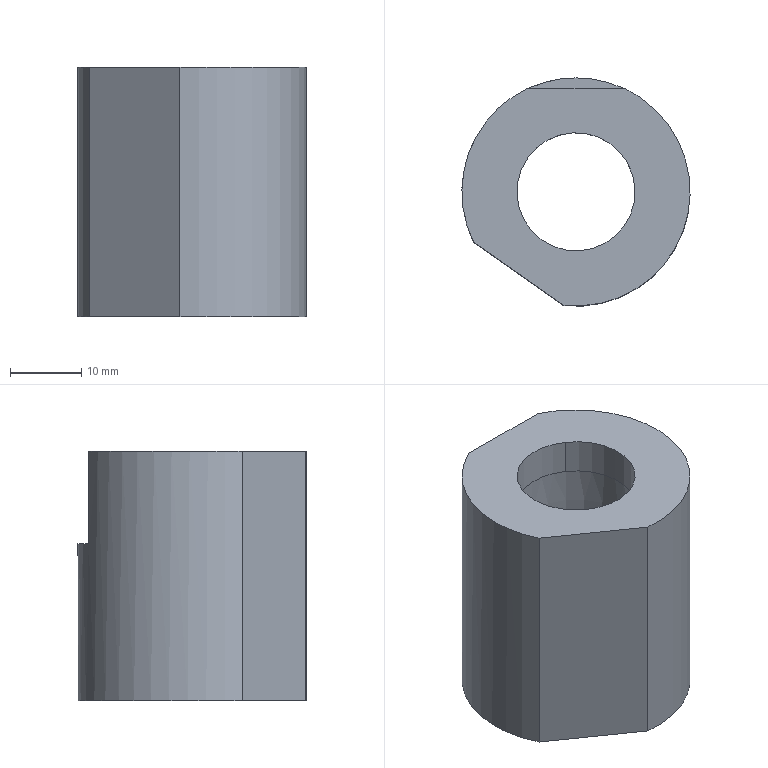Part | STEP file | 1_id4534_x_t | 1 solid | 9 faces | box 32 x 32 x 35 mm | volume 19058 mm3 | plane 5 | cylinder 3 | cone 1 | commonest cylinder face diameters 16.57 x2 32 x1
STEP:
#1=CARTESIAN_POINT('',(3362.815,59.589,-35.));
#2=VERTEX_POINT('',#1);
#3=CARTESIAN_POINT('',(3350.125,68.475,-35.));
#4=VERTEX_POINT('',#3);
#5=CARTESIAN_POINT('',(3356.47,64.032,-35.));
#6=DIRECTION('',(-0.8192,0.5736,0.));
#7=VECTOR('',#6,1.);
#8=LINE('',#5,#7);
#9=EDGE_CURVE('',#2,#4,#8,.T.);
#10=ORIENTED_EDGE('',*,*,#9,.T.);
#11=CARTESIAN_POINT('',(3364.5,75.5,-35.));
#12=DIRECTION('',(0.,0.,1.));
#13=DIRECTION('',(-1.,0.,0.));
#14=AXIS2_PLACEMENT_3D('',#11,#12,#13);
#15=CIRCLE('',#14,16.);
#16=EDGE_CURVE('',#2,#4,#15,.T.);
#17=ORIENTED_EDGE('',*,*,#16,.F.);
#18=EDGE_LOOP('',(#10,#17));
#19=FACE_BOUND('',#18,.T.);
#20=CARTESIAN_POINT('',(3355.43,75.5,-35.));
#21=VERTEX_POINT('',#20);
#22=CARTESIAN_POINT('',(3364.5,75.5,-35.));
#23=DIRECTION('',(0.,0.,1.));
#24=DIRECTION('',(-1.,0.,0.));
#25=AXIS2_PLACEMENT_3D('',#22,#23,#24);
#26=CIRCLE('',#25,9.071);
#27=EDGE_CURVE('',#21,#21,#26,.T.);
#28=ORIENTED_EDGE('',*,*,#27,.T.);
#29=EDGE_LOOP('',(#28));
#30=FACE_BOUND('',#29,.T.);
#31=CARTESIAN_POINT('',(3368.085,80.62,-35.));
#32=DIRECTION('',(0.,0.,-1.));
#33=DIRECTION('',(0.5736,0.8192,0.));
#34=AXIS2_PLACEMENT_3D('',#31,#32,#33);
#35=PLANE('',#34);
#36=ADVANCED_FACE('',(#19,#30),#35,.T.);
#37=CARTESIAN_POINT('',(3362.815,59.589,0.00001741));
#38=VERTEX_POINT('',#37);
#39=CARTESIAN_POINT('',(3373.677,88.607,0.00001741));
#40=VERTEX_POINT('',#39);
#41=CARTESIAN_POINT('',(3364.5,75.5,0.00001741));
#42=DIRECTION('',(0.,0.,1.));
#43=DIRECTION('',(0.8192,-0.5736,0.));
#44=AXIS2_PLACEMENT_3D('',#41,#42,#43);
#45=CIRCLE('',#44,16.);
#46=EDGE_CURVE('',#38,#40,#45,.T.);
#47=ORIENTED_EDGE('',*,*,#46,.F.);
#48=CARTESIAN_POINT('',(3362.815,59.589,-17.5));
#49=DIRECTION('',(0.,0.,-1.));
#50=VECTOR('',#49,1.);
#51=LINE('',#48,#50);
#52=EDGE_CURVE('',#38,#2,#51,.T.);
#53=ORIENTED_EDGE('',*,*,#52,.T.);
#54=ORIENTED_EDGE('',*,*,#16,.T.);
#55=CARTESIAN_POINT('',(3350.125,68.475,0.00001741));
#56=VERTEX_POINT('',#55);
#57=CARTESIAN_POINT('',(3350.125,68.475,-17.5));
#58=DIRECTION('',(0.,0.,1.));
#59=VECTOR('',#58,1.);
#60=LINE('',#57,#59);
#61=EDGE_CURVE('',#4,#56,#60,.T.);
#62=ORIENTED_EDGE('',*,*,#61,.T.);
#63=CARTESIAN_POINT('',(3357.736,90.,0.00001741));
#64=VERTEX_POINT('',#63);
#65=CARTESIAN_POINT('',(3364.5,75.5,0.00001741));
#66=DIRECTION('',(0.,0.,1.));
#67=DIRECTION('',(0.8192,-0.5736,0.));
#68=AXIS2_PLACEMENT_3D('',#65,#66,#67);
#69=CIRCLE('',#68,16.);
#70=EDGE_CURVE('',#64,#56,#69,.T.);
#71=ORIENTED_EDGE('',*,*,#70,.F.);
#72=CARTESIAN_POINT('',(3357.736,90.,-13.));
#73=VERTEX_POINT('',#72);
#74=CARTESIAN_POINT('',(3357.736,90.,-17.5));
#75=DIRECTION('',(0.,0.,1.));
#76=VECTOR('',#75,1.);
#77=LINE('',#74,#76);
#78=EDGE_CURVE('',#73,#64,#77,.T.);
#79=ORIENTED_EDGE('',*,*,#78,.F.);
#80=CARTESIAN_POINT('',(3371.264,90.,-13.));
#81=VERTEX_POINT('',#80);
#82=CARTESIAN_POINT('',(3364.5,75.5,-13.));
#83=DIRECTION('',(0.,0.,1.));
#84=DIRECTION('',(-1.,0.,0.));
#85=AXIS2_PLACEMENT_3D('',#82,#83,#84);
#86=CIRCLE('',#85,16.);
#87=EDGE_CURVE('',#81,#73,#86,.T.);
#88=ORIENTED_EDGE('',*,*,#87,.F.);
#89=CARTESIAN_POINT('',(3371.264,90.,0.00001741));
#90=VERTEX_POINT('',#89);
#91=CARTESIAN_POINT('',(3371.264,90.,-17.5));
#92=DIRECTION('',(0.,0.,-1.));
#93=VECTOR('',#92,1.);
#94=LINE('',#91,#93);
#95=EDGE_CURVE('',#90,#81,#94,.T.);
#96=ORIENTED_EDGE('',*,*,#95,.F.);
#97=CARTESIAN_POINT('',(3364.5,75.5,0.00001741));
#98=DIRECTION('',(0.,0.,1.));
#99=DIRECTION('',(0.8192,-0.5736,0.));
#100=AXIS2_PLACEMENT_3D('',#97,#98,#99);
#101=CIRCLE('',#100,16.);
#102=EDGE_CURVE('',#40,#90,#101,.T.);
#103=ORIENTED_EDGE('',*,*,#102,.F.);
#104=CARTESIAN_POINT('',(3373.677,88.607,-30.));
#105=VERTEX_POINT('',#104);
#106=CARTESIAN_POINT('',(3373.677,88.607,-17.5));
#107=DIRECTION('',(0.,0.,1.));
#108=VECTOR('',#107,1.);
#109=LINE('',#106,#108);
#110=EDGE_CURVE('',#105,#40,#109,.T.);
#111=ORIENTED_EDGE('',*,*,#110,.F.);
#112=ORIENTED_EDGE('',*,*,#110,.T.);
#113=EDGE_LOOP('',(#47,#53,#54,#62,#71,#79,#88,#96,#103,#111,#112));
#114=FACE_OUTER_BOUND('',#113,.T.);
#115=CARTESIAN_POINT('',(3364.5,75.5,-17.5));
#116=DIRECTION('',(0.,0.,1.));
#117=DIRECTION('',(-0.5736,-0.8192,0.));
#118=AXIS2_PLACEMENT_3D('',#115,#116,#117);
#119=CYLINDRICAL_SURFACE('',#118,16.);
#120=ADVANCED_FACE('',(#114),#119,.T.);
#121=CARTESIAN_POINT('',(3368.085,90.,0.00001741));
#122=DIRECTION('',(1.,0.,0.));
#123=VECTOR('',#122,1.);
#124=LINE('',#121,#123);
#125=EDGE_CURVE('',#64,#90,#124,.T.);
#126=ORIENTED_EDGE('',*,*,#125,.F.);
#127=ORIENTED_EDGE('',*,*,#70,.T.);
#128=CARTESIAN_POINT('',(3356.47,64.032,0.00001741));
#129=DIRECTION('',(0.8192,-0.5736,0.));
#130=VECTOR('',#129,1.);
#131=LINE('',#128,#130);
#132=EDGE_CURVE('',#56,#38,#131,.T.);
#133=ORIENTED_EDGE('',*,*,#132,.T.);
#134=ORIENTED_EDGE('',*,*,#46,.T.);
#135=ORIENTED_EDGE('',*,*,#102,.T.);
#136=EDGE_LOOP('',(#126,#127,#133,#134,#135));
#137=FACE_BOUND('',#136,.T.);
#138=CARTESIAN_POINT('',(3359.748,68.713,0.00001741));
#139=VERTEX_POINT('',#138);
#140=CARTESIAN_POINT('',(3369.252,82.287,0.00001741));
#141=VERTEX_POINT('',#140);
#142=CARTESIAN_POINT('',(3364.5,75.5,0.00001741));
#143=DIRECTION('',(0.,0.,-1.));
#144=DIRECTION('',(0.8192,-0.5736,0.));
#145=AXIS2_PLACEMENT_3D('',#142,#143,#144);
#146=CIRCLE('',#145,8.285);
#147=EDGE_CURVE('',#139,#141,#146,.T.);
#148=ORIENTED_EDGE('',*,*,#147,.T.);
#149=CARTESIAN_POINT('',(3364.5,75.5,0.00001741));
#150=DIRECTION('',(0.,0.,-1.));
#151=DIRECTION('',(0.8192,-0.5736,0.));
#152=AXIS2_PLACEMENT_3D('',#149,#150,#151);
#153=CIRCLE('',#152,8.285);
#154=EDGE_CURVE('',#141,#139,#153,.T.);
#155=ORIENTED_EDGE('',*,*,#154,.T.);
#156=EDGE_LOOP('',(#148,#155));
#157=FACE_BOUND('',#156,.T.);
#158=CARTESIAN_POINT('',(3368.085,80.62,0.00001741));
#159=DIRECTION('',(0.,0.,1.));
#160=DIRECTION('',(-0.5736,-0.8192,0.));
#161=AXIS2_PLACEMENT_3D('',#158,#159,#160);
#162=PLANE('',#161);
#163=ADVANCED_FACE('',(#137,#157),#162,.T.);
#164=CARTESIAN_POINT('',(3369.252,82.287,-5.));
#165=VERTEX_POINT('',#164);
#166=CARTESIAN_POINT('',(3359.748,68.713,-5.));
#167=VERTEX_POINT('',#166);
#168=CARTESIAN_POINT('',(3364.5,75.5,-5.));
#169=DIRECTION('',(0.,0.,1.));
#170=DIRECTION('',(0.8192,-0.5736,0.));
#171=AXIS2_PLACEMENT_3D('',#168,#169,#170);
#172=CIRCLE('',#171,8.285);
#173=EDGE_CURVE('',#165,#167,#172,.T.);
#174=ORIENTED_EDGE('',*,*,#173,.F.);
#175=CARTESIAN_POINT('',(3369.252,82.287,-3.));
#176=DIRECTION('',(0.,0.,-1.));
#177=VECTOR('',#176,1.);
#178=LINE('',#175,#177);
#179=EDGE_CURVE('',#141,#165,#178,.T.);
#180=ORIENTED_EDGE('',*,*,#179,.F.);
#181=ORIENTED_EDGE('',*,*,#147,.F.);
#182=CARTESIAN_POINT('',(3359.748,68.713,-3.));
#183=DIRECTION('',(0.,0.,1.));
#184=VECTOR('',#183,1.);
#185=LINE('',#182,#184);
#186=EDGE_CURVE('',#167,#139,#185,.T.);
#187=ORIENTED_EDGE('',*,*,#186,.F.);
#188=EDGE_LOOP('',(#174,#180,#181,#187));
#189=FACE_OUTER_BOUND('',#188,.T.);
#190=CARTESIAN_POINT('',(3364.5,75.5,-3.));
#191=DIRECTION('',(0.,0.,-1.));
#192=DIRECTION('',(-0.5736,-0.8192,0.));
#193=AXIS2_PLACEMENT_3D('',#190,#191,#192);
#194=CYLINDRICAL_SURFACE('',#193,8.285);
#195=ADVANCED_FACE('',(#189),#194,.F.);
#196=CARTESIAN_POINT('',(3364.5,75.5,-5.));
#197=DIRECTION('',(0.,0.,1.));
#198=DIRECTION('',(0.8192,-0.5736,0.));
#199=AXIS2_PLACEMENT_3D('',#196,#197,#198);
#200=CIRCLE('',#199,8.285);
#201=EDGE_CURVE('',#167,#165,#200,.T.);
#202=ORIENTED_EDGE('',*,*,#201,.F.);
#203=ORIENTED_EDGE('',*,*,#186,.T.);
#204=ORIENTED_EDGE('',*,*,#154,.F.);
#205=ORIENTED_EDGE('',*,*,#179,.T.);
#206=EDGE_LOOP('',(#202,#203,#204,#205));
#207=FACE_OUTER_BOUND('',#206,.T.);
#208=CARTESIAN_POINT('',(3364.5,75.5,-3.));
#209=DIRECTION('',(0.,0.,-1.));
#210=DIRECTION('',(-0.5736,-0.8192,0.));
#211=AXIS2_PLACEMENT_3D('',#208,#209,#210);
#212=CYLINDRICAL_SURFACE('',#211,8.285);
#213=ADVANCED_FACE('',(#207),#212,.F.);
#214=ORIENTED_EDGE('',*,*,#9,.F.);
#215=ORIENTED_EDGE('',*,*,#52,.F.);
#216=ORIENTED_EDGE('',*,*,#132,.F.);
#217=ORIENTED_EDGE('',*,*,#61,.F.);
#218=EDGE_LOOP('',(#214,#215,#216,#217));
#219=FACE_OUTER_BOUND('',#218,.T.);
#220=CARTESIAN_POINT('',(3356.47,64.032,-32.5));
#221=DIRECTION('',(-0.5736,-0.8192,0.));
#222=DIRECTION('',(0.,0.,-1.));
#223=AXIS2_PLACEMENT_3D('',#220,#221,#222);
#224=PLANE('',#223);
#225=ADVANCED_FACE('',(#219),#224,.T.);
#226=ORIENTED_EDGE('',*,*,#27,.F.);
#227=EDGE_LOOP('',(#226));
#228=FACE_BOUND('',#227,.T.);
#229=ORIENTED_EDGE('',*,*,#173,.T.);
#230=ORIENTED_EDGE('',*,*,#201,.T.);
#231=EDGE_LOOP('',(#229,#230));
#232=FACE_BOUND('',#231,.T.);
#233=CARTESIAN_POINT('',(3364.5,75.5,-5.));
#234=DIRECTION('',(0.,0.,-1.));
#235=DIRECTION('',(0.8192,-0.5736,0.));
#236=AXIS2_PLACEMENT_3D('',#233,#234,#235);
#237=CONICAL_SURFACE('',#236,8.285,1.5);
#238=ADVANCED_FACE('',(#228,#232),#237,.F.);
#239=ORIENTED_EDGE('',*,*,#87,.T.);
#240=CARTESIAN_POINT('',(3364.5,90.,-13.));
#241=DIRECTION('',(-1.,0.,0.));
#242=VECTOR('',#241,1.);
#243=LINE('',#240,#242);
#244=EDGE_CURVE('',#81,#73,#243,.T.);
#245=ORIENTED_EDGE('',*,*,#244,.F.);
#246=EDGE_LOOP('',(#239,#245));
#247=FACE_OUTER_BOUND('',#246,.T.);
#248=CARTESIAN_POINT('',(3364.5,98.,-13.));
#249=DIRECTION('',(0.,0.,-1.));
#250=DIRECTION('',(0.,-1.,0.));
#251=AXIS2_PLACEMENT_3D('',#248,#249,#250);
#252=PLANE('',#251);
#253=ADVANCED_FACE('',(#247),#252,.F.);
#254=ORIENTED_EDGE('',*,*,#78,.T.);
#255=ORIENTED_EDGE('',*,*,#125,.T.);
#256=ORIENTED_EDGE('',*,*,#95,.T.);
#257=ORIENTED_EDGE('',*,*,#244,.T.);
#258=EDGE_LOOP('',(#254,#255,#256,#257));
#259=FACE_OUTER_BOUND('',#258,.T.);
#260=CARTESIAN_POINT('',(3364.5,90.,-1.));
#261=DIRECTION('',(0.,-1.,0.));
#262=DIRECTION('',(0.,0.,1.));
#263=AXIS2_PLACEMENT_3D('',#260,#261,#262);
#264=PLANE('',#263);
#265=ADVANCED_FACE('',(#259),#264,.F.);
#266=CLOSED_SHELL('',(#36,#120,#163,#195,#213,#225,#238,#253,#265));
#267=MANIFOLD_SOLID_BREP('',#266);
#268=(LENGTH_UNIT()NAMED_UNIT(*)SI_UNIT(.MILLI.,.METRE.));
#269=UNCERTAINTY_MEASURE_WITH_UNIT(LENGTH_MEASURE(0.00002),#268,'','');
#270=(NAMED_UNIT(*)PLANE_ANGLE_UNIT()SI_UNIT($,.RADIAN.));
#271=PLANE_ANGLE_MEASURE_WITH_UNIT(PLANE_ANGLE_MEASURE(0.01745),#270);
#272=DIMENSIONAL_EXPONENTS(0.,0.,0.,0.,0.,0.,0.);
#273=(CONVERSION_BASED_UNIT('DEGREE',#271)NAMED_UNIT(#272)PLANE_ANGLE_UNIT());
#274=(NAMED_UNIT(*)SI_UNIT($,.STERADIAN.)SOLID_ANGLE_UNIT());
#275=(GEOMETRIC_REPRESENTATION_CONTEXT(3)GLOBAL_UNCERTAINTY_ASSIGNED_CONTEXT((#269))GLOBAL_UNIT_ASSIGNED_CONTEXT((#268,#273,#274))REPRESENTATION_CONTEXT('',''));
#276=ADVANCED_BREP_SHAPE_REPRESENTATION('',(#267),#275);